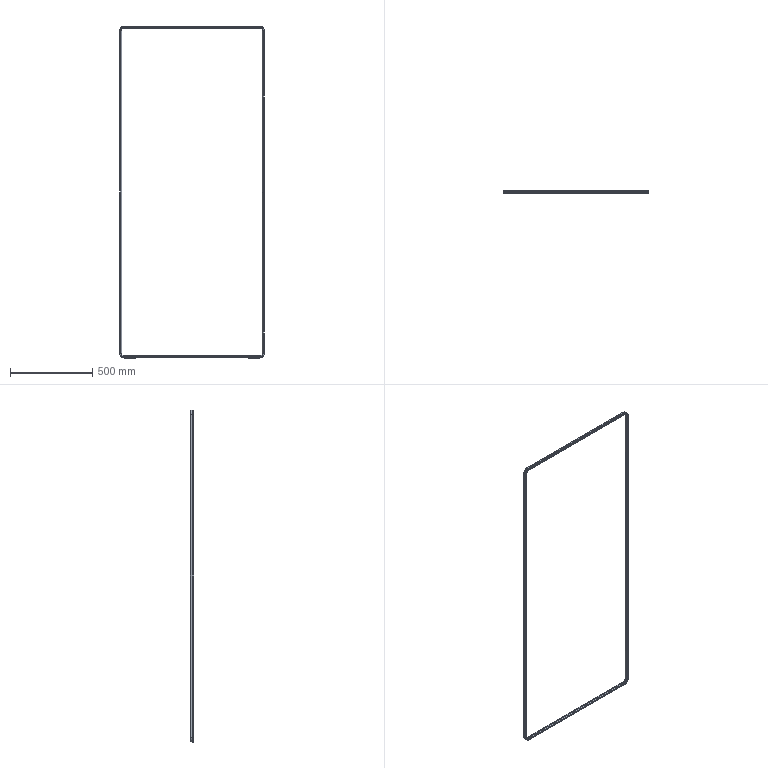Part | STEP file | 750038419 | 1 solid | 366 faces | box 881.505 x 20.12 x 2022 mm | volume 451078 mm3 | cylinder 145 | spline 134 | plane 55 | cone 32 | commonest cylinder face diameters 0.6 x60 1 x40 2.05 x18 0.4 x15 5 x6 9.1 x6